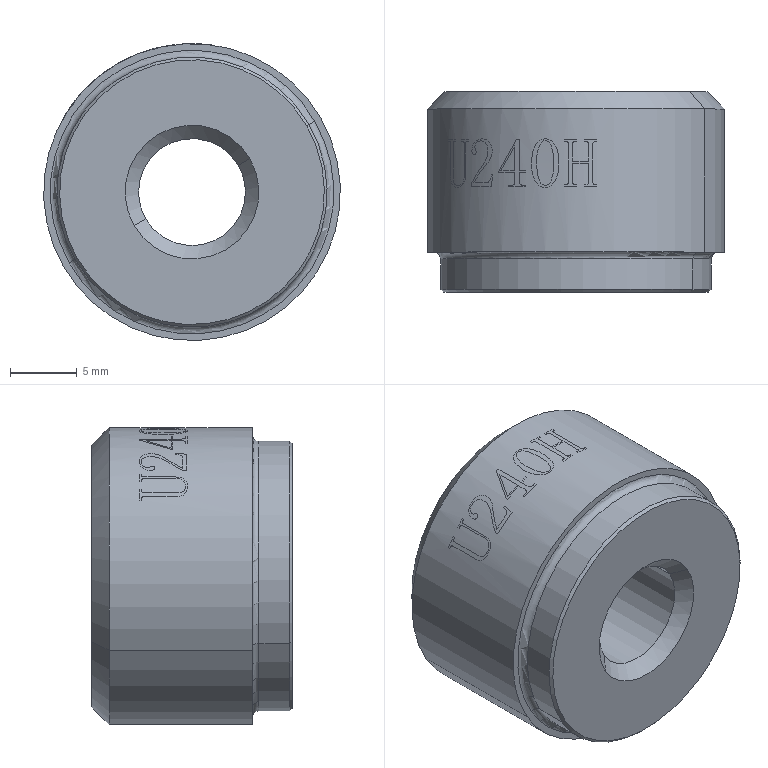Part | SolidWorks | features BaseBody 1 | 1 solid | 26 faces | box 22.2 x 15 x 22.2 mm | volume 4784 mm3 | cylinder 13 | cone 8 | plane 3 | torus 2 | commonest cylinder face diameters 22.2 x9 8 x2 20.2 x2